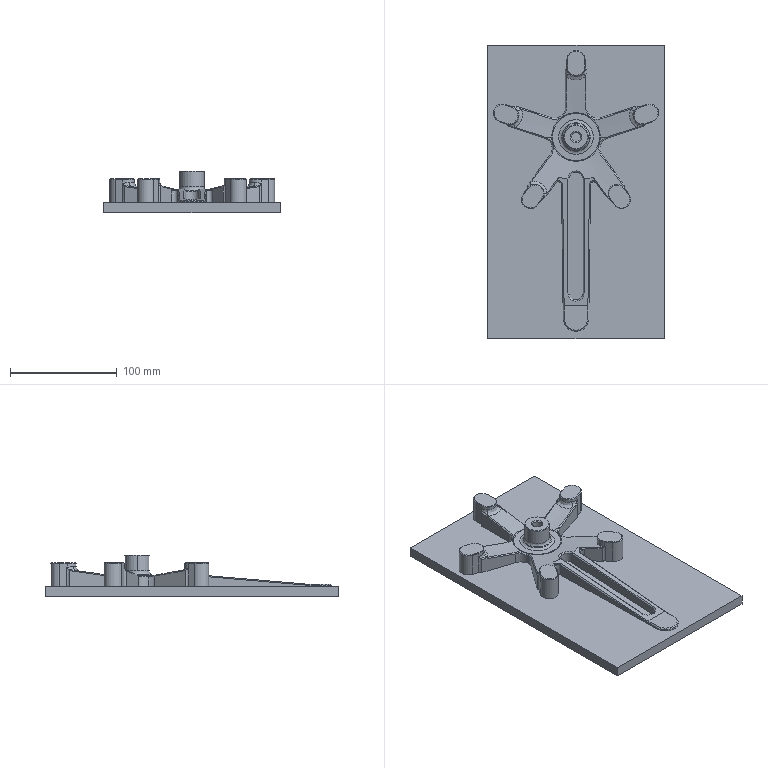NC program | NX | posted with a generic post | part box 165 x 275 x 39 mm
Lines 61374 to 62133 of 70117:
(CONTOUR_AREA , TOOL : D6R3)
N122728 M6
N122730 G54
N122732 G17 G0 G90 X-8.166 Y-25.337 S0 M3
N122734 G43 Z30. H0
N122736 Z-15.6
N122738 G94 G1 Z-15.879 F250.
N122740 X-8.132 Y-25.323 Z-16.661
N122742 X-7.912 Y-25.231 Z-17.407
N122744 X-7.52 Y-25.069 Z-18.066
N122746 X-6.985 Y-24.847 Z-18.592
N122748 X-6.343 Y-24.579 Z-18.951
N122750 X-5.636 Y-24.286 Z-19.118
N122752 X-5.524 Y-24.239 Z-19.128
N122754 X-5.17 Y-24.108 Z-19.157
N122756 X-6.054 Y-23.865 Z-19.162
N122758 X-6.08 Y-23.916 Z-19.154
N122760 X-6.134 Y-24.015 Z-19.139
N122762 X-5.636 Y-24.286 Z-19.118
N122764 X-5.67 Y-24.841 Z-19.038
N122766 X-4.418 Y-24.384 Z-19.139
N122768 X-3.506 Y-24.128 Z-19.197
N122770 X-2.576 Y-23.949 Z-19.239
N122772 X-4.835 Y-23.681 Z-19.228
N122774 X-5.038 Y-23.625 Z-19.229
N122776 X-6.312 Y-23.276 Z-19.235
N122778 X-6.522 Y-23.681 Z-19.171
N122780 X-6.82 Y-24.225 Z-19.084
N122782 X-5.67 Y-24.841 Z-19.038
N122784 X-5.866 Y-25.306 Z-18.967
N122786 X-5.708 Y-25.398 Z-18.959
N122788 X-4.262 Y-24.859 Z-19.075
N122790 X-3.03 Y-24.535 Z-19.148
N122792 X-1.768 Y-24.361 Z-19.191
N122794 X0.969 Y-24.263 Z-19.211
N122796 X2.152 Y-24.397 Z-19.181
N122798 X3.437 Y-24.623 Z-19.128
N122800 X4.684 Y-25.004 Z-19.044
N122802 X5.644 Y-25.399 Z-18.96
N122804 X6.581 Y-24.874 Z-19.002
N122806 X7.544 Y-24.399 Z-19.03
N122808 X7.076 Y-23.547 Z-19.167
N122810 X6.607 Y-22.696 Z-19.304
N122812 X5.938 Y-22.896 Z-19.302
N122814 X4.869 Y-23.088 Z-19.311
N122816 X5.046 Y-24.072 Z-19.166
N122818 X5.05 Y-24.073
N122820 X5.569 Y-24.287 Z-19.12
N122822 X6.163 Y-23.964 Z-19.145
N122824 X6.117 Y-23.88 Z-19.158
N122826 X5.046 Y-24.072 Z-19.166
N122828 X4.957 Y-23.58 Z-19.238
N122830 X2.752 Y-23.976 Z-19.233
N122832 X3.823 Y-24.205 Z-19.179
N122834 X4.867 Y-24.539 Z-19.105
N122836 X5.605 Y-24.843 Z-19.04
N122838 X6.851 Y-24.176 Z-19.089
N122840 X6.363 Y-23.29 Z-19.231
N122842 X6.054 Y-23.383 Z-19.23
N122844 X4.957 Y-23.58 Z-19.238
N122846 X4.869 Y-23.088 Z-19.311
N122848 X2.114 Y-23.582 Z-19.299
N122850 X-0.73 Y-23.633 Z-19.303
N122852 X-2.734 Y-23.411 Z-19.314
N122854 X-4.739 Y-23.189 Z-19.3
N122856 X-6.579 Y-22.685 Z-19.307
N122858 X-7.046 Y-23.566 Z-19.166
N122860 X-7.512 Y-24.447 Z-19.025
N122862 X-5.866 Y-25.306 Z-18.967
N122864 X-6.117 Y-25.738 Z-18.897
N122866 X-5.749 Y-25.957 Z-18.879
N122868 X-4.106 Y-25.335 Z-19.012
N122870 X-2.937 Y-25.027 Z-19.079
N122872 X-1.74 Y-24.86 Z-19.119
N122874 X0.95 Y-24.764 Z-19.139
N122876 X2.096 Y-24.894 Z-19.11
N122878 X3.316 Y-25.108 Z-19.061
N122880 X4.501 Y-25.47 Z-18.983
N122882 X5.687 Y-25.958 Z-18.88
N122884 X6.942 Y-25.25 Z-18.936
N122886 X8.244 Y-24.634 Z-18.966
N122888 X7.547 Y-23.368 Z-19.172
N122890 X6.85 Y-22.101 Z-19.376
N122892 X5.822 Y-22.408 Z-19.374
N122894 X3.945 Y-22.745 Z-19.384
N122896 X2.067 Y-23.082 Z-19.371
N122898 X-0.712 Y-23.134 Z-19.376
N122900 X-1.104 Y-23.117
N122902 X-4.643 Y-22.697 Z-19.372
N122904 X-6.847 Y-22.093 Z-19.378
N122906 X-7.497 Y-23.328 Z-19.179
N122908 X-8.146 Y-24.563 Z-18.981
N122910 X-8.215 Y-24.68 Z-18.962
N122912 X-7.15 Y-25.178 Z-18.938
N122914 X-6.117 Y-25.738 Z-18.897
N122916 X-6.367 Y-26.171 Z-18.828
N122918 X-5.794 Y-26.517 Z-18.798
N122920 X-3.951 Y-25.81 Z-18.947
N122922 X-2.844 Y-25.518 Z-19.01
N122924 X-1.711 Y-25.36 Z-19.047
N122926 X0.93 Y-25.265 Z-19.067
N122928 X2.04 Y-25.391 Z-19.039
N122930 X3.196 Y-25.594 Z-18.993
N122932 X4.319 Y-25.935 Z-18.921
N122934 X5.733 Y-26.517 Z-18.8
N122936 X6.511 Y-26.052 Z-18.84
N122938 X7.31 Y-25.623 Z-18.87
N122940 X8.962 Y-24.879 Z-18.899
N122942 X8.289 Y-23.707 Z-19.091
N122944 X7.616 Y-22.534 Z-19.283
N122946 X7.336 Y-21.956 Z-19.375
N122948 X7.121 Y-21.499 Z-19.448
N122950 X5.706 Y-21.921 Z-19.447
N122952 X3.863 Y-22.252 Z-19.456
N122954 X2.021 Y-22.583 Z-19.444
N122956 X-0.695 Y-22.634 Z-19.448
N122958 X-1.064 Y-22.618
N122960 X-4.547 Y-22.205 Z-19.445
N122962 X-7.121 Y-21.499 Z-19.447
N122964 X-7.327 Y-21.937 Z-19.378
N122966 X-8.646 Y-24.425 Z-18.976
N122968 X-8.908 Y-24.868 Z-18.903
N122970 X-8.941 Y-24.92 Z-18.895
N122972 X-7.631 Y-25.498 Z-18.874
N122974 X-6.367 Y-26.171 Z-18.828
N122976 X-6.618 Y-26.603 Z-18.759
N122978 X-5.842 Y-27.079 Z-18.717
N122980 X-4.609 Y-26.566 Z-18.824
N122982 X-4.273 Y-26.442 Z-18.85
N122984 X-3.795 Y-26.285 Z-18.883
N122986 X-2.751 Y-26.009 Z-18.941
N122988 X-1.682 Y-25.859 Z-18.976
N122990 X0.911 Y-25.766 Z-18.995
N122992 X1.983 Y-25.888 Z-18.969
N122994 X3.076 Y-26.079 Z-18.926
N122996 X4.137 Y-26.401 Z-18.859
N122998 X5.784 Y-27.079 Z-18.719
N123000 X7.052 Y-26.324 Z-18.782
N123002 X8.374 Y-25.669 Z-18.819
N123004 X9.743 Y-25.119 Z-18.827
N123006 X9.059 Y-24.151 Z-18.993
N123008 X7.785 Y-21.738 Z-19.384
N123010 X7.58 Y-21.3 Z-19.453
N123012 X7.385 Y-20.857 Z-19.499
N123014 X6.98 Y-21.019 Z-19.498
N123016 X5.59 Y-21.434
N123018 X4.686 Y-21.596 Z-19.5
N123020 X4.093 Y-21.703
N123022 X3.697 Y-21.774
N123024 X2.878 Y-21.921 Z-19.499
N123026 X1.974 Y-22.083 Z-19.497
N123028 X-0.678 Y-22.134 Z-19.498
N123030 X-1.024 Y-22.12
N123032 X-4.451 Y-21.712 Z-19.497
N123034 X-6.983 Y-21.019 Z-19.498
N123036 X-7.389 Y-20.869
N123038 X-7.578 Y-21.296 Z-19.454
N123040 X-7.777 Y-21.718 Z-19.387
N123042 X-9.015 Y-24.067 Z-19.006
N123044 X-9.334 Y-24.606 Z-18.917
N123046 X-9.693 Y-25.169 Z-18.823
N123048 X-8.123 Y-25.817 Z-18.809
N123050 X-6.618 Y-26.603 Z-18.759
N123052 X-6.869 Y-27.036 Z-18.69
N123054 X-5.884 Y-27.65 Z-18.636
N123056 X-4.108 Y-26.914 Z-18.786
N123058 X-3.639 Y-26.76 Z-18.818
N123060 X-2.657 Y-26.501 Z-18.872
N123062 X-1.652 Y-26.358 Z-18.904
N123064 X0.892 Y-26.267 Z-18.922
N123066 X1.927 Y-26.385 Z-18.898
N123068 X2.956 Y-26.564 Z-18.858
N123070 X3.955 Y-26.867 Z-18.796
N123072 X5.838 Y-27.642 Z-18.638
N123074 X6.574 Y-27.174 Z-18.68
N123076 X7.331 Y-26.741 Z-18.714
N123078 X8.903 Y-25.984 Z-18.751
N123080 X10.538 Y-25.378 Z-18.749
N123082 X10.011 Y-24.632 Z-18.878
N123084 X9.484 Y-23.886 Z-19.007
N123086 X8.235 Y-21.52 Z-19.391
N123088 X7.935 Y-20.869 Z-19.488
N123090 X7.864 Y-20.705 Z-19.498
N123092 X7.846 Y-20.664 Z-19.499
N123094 X7.66 Y-20.208 Z-19.5
N123096 X6.815 Y-20.547
N123098 X5.474 Y-20.947
N123100 X1.928 Y-21.584
N123102 X-0.661 Y-21.634
N123104 X-0.984 Y-21.621
N123106 X-4.355 Y-21.22
N123108 X-6.83 Y-20.542
N123110 X-7.668 Y-20.232
N123112 X-7.799 Y-20.553
N123114 X-7.832 Y-20.633
N123116 X-7.841 Y-20.653
N123118 X-7.849 Y-20.673 Z-19.499
N123120 X-7.866 Y-20.713 Z-19.498
N123122 X-7.935 Y-20.871 Z-19.488
N123124 X-8.227 Y-21.5 Z-19.394
N123126 X-9.449 Y-23.82 Z-19.017
N123128 X-10.466 Y-25.432 Z-18.746
N123130 X-8.625 Y-26.138 Z-18.743
N123132 X-6.869 Y-27.036 Z-18.69
N123134 X-7.12 Y-27.468 Z-18.62
N123136 X-5.917 Y-28.232 Z-18.552
N123138 X-5.557 Y-28.043 Z-18.589
N123140 X-4.243 Y-27.497 Z-18.7
N123142 X-3.943 Y-27.386 Z-18.722
N123144 X-3.483 Y-27.235 Z-18.753
N123146 X-2.564 Y-26.992 Z-18.802
N123148 X-1.622 Y-26.857 Z-18.832
N123150 X0.872 Y-26.768 Z-18.85
N123152 X1.871 Y-26.881 Z-18.827
N123154 X2.836 Y-27.05 Z-18.79
N123156 X3.773 Y-27.333 Z-18.733
N123158 X5.897 Y-28.207 Z-18.556
N123160 X6.742 Y-27.657 Z-18.607
N123162 X7.616 Y-27.156 Z-18.645
N123164 X9.441 Y-26.303 Z-18.682
N123166 X11.35 Y-25.659 Z-18.666
N123168 X10.636 Y-24.652 Z-18.841
N123170 X9.922 Y-23.645 Z-19.015
N123172 X8.685 Y-21.301 Z-19.396
N123174 X8.484 Y-20.872 Z-19.464
N123176 X8.387 Y-20.655 Z-19.492
N123178 X8.34 Y-20.547 Z-19.497
N123180 X8.317 Y-20.492 Z-19.499
N123182 X7.948 Y-19.554 Z-19.5
N123184 X6.65 Y-20.074
N123186 X5.358 Y-20.46
N123188 X1.881 Y-21.084
N123190 X-0.644 Y-21.135
N123192 X-0.944 Y-21.122
N123194 X-4.259 Y-20.728
N123196 X-6.677 Y-20.066
N123198 X-7.958 Y-19.59
N123200 X-8.295 Y-20.444
N123202 X-8.307 Y-20.471
N123204 X-8.318 Y-20.497 Z-19.499
N123206 X-8.341 Y-20.55 Z-19.497
N123208 X-8.387 Y-20.655 Z-19.492
N123210 X-8.481 Y-20.865 Z-19.466
N123212 X-8.676 Y-21.281 Z-19.399
N123214 X-9.884 Y-23.572 Z-19.027
N123216 X-10.954 Y-25.261 Z-18.742
N123218 X-11.277 Y-25.709 Z-18.664
N123220 X-9.844 Y-26.179 Z-18.679
N123222 X-8.455 Y-26.766 Z-18.664
N123224 X-7.12 Y-27.468 Z-18.62
N123226 X-7.371 Y-27.901 Z-18.55
N123228 X-5.955 Y-28.816 Z-18.468
N123230 X-5.344 Y-28.496 Z-18.531
N123232 X-4.06 Y-27.962 Z-18.638
N123234 X-3.778 Y-27.858 Z-18.658
N123236 X-3.327 Y-27.71 Z-18.687
N123238 X-2.47 Y-27.483 Z-18.733
N123240 X-1.592 Y-27.357 Z-18.761
N123242 X0.853 Y-27.269 Z-18.778
N123244 X1.815 Y-27.378 Z-18.755
N123246 X2.716 Y-27.535 Z-18.722
N123248 X3.592 Y-27.799 Z-18.67
N123250 X5.762 Y-28.692 Z-18.492
N123252 X5.926 Y-28.797 Z-18.472
N123254 X6.64 Y-28.311 Z-18.518
N123256 X7.377 Y-27.861 Z-18.556
N123258 X8.913 Y-27.072 Z-18.602
N123260 X10.519 Y-26.437 Z-18.609
N123262 X12.18 Y-25.964 Z-18.576
N123264 X11.263 Y-24.672 Z-18.801
N123266 X10.347 Y-23.38 Z-19.026
N123268 X9.135 Y-21.083 Z-19.4
N123270 X8.886 Y-20.547 Z-19.482
N123272 X8.768 Y-20.277 Z-19.5
N123274 X8.655 Y-20.004
N123276 X8.249 Y-18.895
N123278 X6.485 Y-19.601
N123280 X5.242 Y-19.973
N123282 X1.834 Y-20.584
N123284 X-0.626 Y-20.635
N123286 X-0.904 Y-20.623
N123288 X-4.163 Y-20.236
N123290 X-6.524 Y-19.589
N123292 X-8.252 Y-18.915
N123294 X-8.654 Y-20.003
N123296 X-8.765 Y-20.271
N123298 X-8.772 Y-20.288 Z-19.499
N123300 X-8.779 Y-20.304
N123302 X-8.794 Y-20.338 Z-19.497
N123304 X-8.822 Y-20.404 Z-19.495
N123306 X-8.881 Y-20.537 Z-19.483
N123308 X-9.126 Y-21.062 Z-19.403
N123310 X-10.318 Y-23.324 Z-19.035
N123312 X-11.364 Y-24.975 Z-18.755
N123314 X-12.108 Y-26.009 Z-18.575
N123316 X-10.47 Y-26.485 Z-18.605
N123318 X-8.886 Y-27.117 Z-18.597
N123320 X-7.371 Y-27.901 Z-18.55
N123322 X-7.623 Y-28.334 Z-18.48
N123324 X-5.976 Y-29.423 Z-18.382
N123326 X-5.704 Y-29.249 Z-18.414
N123328 X-5.132 Y-28.949 Z-18.472
N123330 X-3.877 Y-28.428 Z-18.575
N123332 X-3.613 Y-28.33 Z-18.594
N123334 X-3.172 Y-28.185 Z-18.622
N123336 X-2.376 Y-27.974 Z-18.664
N123338 X-1.562 Y-27.856 Z-18.689
N123340 X0.834 Y-27.77 Z-18.706
N123342 X1.758 Y-27.875 Z-18.684
N123344 X2.596 Y-28.021 Z-18.654
N123346 X3.411 Y-28.265 Z-18.606
N123348 X5.53 Y-29.137 Z-18.435
N123350 X5.945 Y-29.404 Z-18.386
N123352 X6.742 Y-28.842 Z-18.44
N123354 X7.57 Y-28.327 Z-18.483
N123356 X9.308 Y-27.443 Z-18.533
N123358 X11.136 Y-26.763 Z-18.531
N123360 X13.029 Y-26.297 Z-18.48
N123362 X10.785 Y-23.139 Z-19.031
N123364 X9.585 Y-20.865 Z-19.402
N123366 X9.314 Y-20.278 Z-19.489
N123368 X9.249 Y-20.13 Z-19.498
N123370 X9.233 Y-20.093 Z-19.499
N123372 G2 X8.566 Y-18.229 R16.959
N123374 G1 X6.321 Y-19.129 Z-19.5
N123376 X5.126 Y-19.486
N123378 X1.788 Y-20.085
N123380 X-0.609 Y-20.135
N123382 X-0.864 Y-20.125
N123384 X-4.067 Y-19.744
N123386 X-6.371 Y-19.113
N123388 X-8.048 Y-18.459
N123390 X-8.562 Y-18.229
N123392 X-8.624 Y-18.439
N123394 X-9.054 Y-19.659
N123396 X-9.215 Y-20.052
N123398 X-9.223 Y-20.071
N123400 X-9.239 Y-20.108 Z-19.498
N123402 X-9.304 Y-20.256 Z-19.492
N123404 X-9.576 Y-20.844 Z-19.406
N123406 X-10.752 Y-23.076 Z-19.041
N123408 X-11.774 Y-24.688 Z-18.768
N123410 X-12.96 Y-26.337 Z-18.479
N123412 X-11.11 Y-26.801 Z-18.528
N123414 X-9.324 Y-27.47
N123416 X-7.623 Y-28.334 Z-18.48
N123418 X-7.874 Y-28.767 Z-18.411
N123420 X-6.916 Y-29.368 Z-18.361
N123422 X-6.001 Y-30.034 Z-18.295
N123424 X-5.452 Y-29.681 Z-18.36
N123426 X-4.92 Y-29.403 Z-18.413
N123428 X-3.016 Y-28.66 Z-18.556
N123430 X-2.282 Y-28.465 Z-18.594
N123432 X-1.531 Y-28.355 Z-18.617
N123434 X0.814 Y-28.271 Z-18.633
N123436 X1.702 Y-28.372 Z-18.613
N123438 X2.477 Y-28.506 Z-18.586
N123440 X3.23 Y-28.731 Z-18.543
N123442 X5.298 Y-29.582 Z-18.378
N123444 X5.969 Y-30.014 Z-18.299
N123446 X6.67 Y-29.496 Z-18.351
N123448 X7.396 Y-29.016 Z-18.394
N123450 X8.921 Y-28.173 Z-18.45
N123452 X10.525 Y-27.495 Z-18.466
N123454 X12.192 Y-26.989 Z-18.441
N123456 X13.902 Y-26.662 Z-18.376
N123458 X11.21 Y-22.873 Z-19.039
N123460 X10.034 Y-20.646 Z-19.403
N123462 X9.772 Y-20.078 Z-19.488
N123464 X9.709 Y-19.934 Z-19.497
N123466 X9.679 Y-19.862 Z-19.5
N123468 X9.53 Y-19.499
N123470 X9.115 Y-18.317
N123472 X8.876 Y-17.518
N123474 X8.627 Y-17.666
N123476 X6.156 Y-18.656
N123478 X5.01 Y-18.998
N123480 X1.741 Y-19.585
N123482 X-0.592 Y-19.636
N123484 X-0.824 Y-19.626
N123486 X-3.97 Y-19.252
N123488 X-6.218 Y-18.636
N123490 X-7.546 Y-18.136
N123492 X-8.872 Y-17.516
N123494 G2 X-9.676 Y-19.858 R17.69
N123496 G1 X-9.684 Y-19.876 Z-19.499
N123498 X-9.699 Y-19.912 Z-19.498
N123500 X-9.762 Y-20.056 Z-19.491
N123502 X-10.025 Y-20.625 Z-19.406
N123504 X-11.187 Y-22.829 Z-19.047
N123506 X-12.184 Y-24.402 Z-18.779
N123508 X-13.839 Y-26.696 Z-18.375
N123510 X-12.28 Y-26.996 Z-18.435
N123512 X-10.757 Y-27.444 Z-18.461
N123514 X-9.284 Y-28.036 Z-18.453
N123516 X-7.874 Y-28.767 Z-18.411
N123518 X-8.125 Y-29.199 Z-18.341
N123520 X-7.05 Y-29.882 Z-18.284
N123522 X-6.032 Y-30.648 Z-18.207
N123524 X-5.201 Y-30.114 Z-18.305
N123526 X-4.707 Y-29.856 Z-18.353
N123528 X-2.86 Y-29.135 Z-18.49
N123530 X-2.188 Y-28.956 Z-18.524
N123532 X-1.499 Y-28.854 Z-18.545
N123534 X0.795 Y-28.772 Z-18.561
N123536 X1.646 Y-28.869 Z-18.542
N123538 X2.357 Y-28.992 Z-18.517
N123540 X3.049 Y-29.198 Z-18.478
N123542 X5.065 Y-30.027 Z-18.32
N123544 X6.001 Y-30.629 Z-18.21
N123546 X6.765 Y-30.042 Z-18.271
N123548 X7.563 Y-29.501 Z-18.32
N123550 X9.25 Y-28.569 Z-18.381
N123552 X11.036 Y-27.846 Z-18.392
N123554 X12.895 Y-27.342 Z-18.352
N123556 X14.802 Y-27.065 Z-18.263
N123558 X11.634 Y-22.607 Z-19.046
N123560 X10.484 Y-20.428 Z-19.402
N123562 X10.23 Y-19.877 Z-19.485
N123564 X10.169 Y-19.738 Z-19.496
N123566 X10.139 Y-19.668 Z-19.499
N123568 G2 X9.171 Y-16.76 R19.731
N123570 G1 X8.404 Y-17.217 Z-19.5
N123572 X5.991 Y-18.184
N123574 X4.894 Y-18.511
N123576 X1.695 Y-19.085
N123578 X-0.784 Y-19.127
N123580 X-3.874 Y-18.76
N123582 X-6.065 Y-18.16
N123584 X-7.345 Y-17.678
N123586 X-8.461 Y-17.179
N123588 X-9.168 Y-16.758
N123590 X-9.581 Y-18.148
N123592 X-9.985 Y-19.294
N123594 X-10.122 Y-19.628
N123596 X-10.129 Y-19.646 Z-19.499
N123598 X-10.159 Y-19.716 Z-19.497
N123600 X-10.22 Y-19.855 Z-19.488
N123602 X-10.475 Y-20.406 Z-19.406
N123604 X-11.621 Y-22.581 Z-19.05
N123606 X-12.594 Y-24.116 Z-18.789
N123608 X-13.67 Y-25.605 Z-18.526
N123610 X-14.746 Y-27.094 Z-18.263
N123612 X-13.014 Y-27.345 Z-18.344
N123614 X-11.32 Y-27.784 Z-18.385
N123616 X-9.684 Y-28.404 Z-18.384
N123618 X-8.125 Y-29.199 Z-18.341
N123620 X-8.377 Y-29.632 Z-18.271
N123622 X-7.182 Y-30.401 Z-18.207
N123624 X-6.062 Y-31.275 Z-18.117
N123626 X-5.929 Y-31.176 Z-18.135
N123628 X-4.949 Y-30.547 Z-18.249
N123630 X-4.495 Y-30.309 Z-18.293
N123632 X-2.704 Y-29.61 Z-18.424
N123634 X-2.093 Y-29.447 Z-18.455
N123636 X-1.467 Y-29.353 Z-18.474
N123638 X0.776 Y-29.273 Z-18.489
N123640 X1.589 Y-29.365 Z-18.471
N123642 X2.238 Y-29.477 Z-18.449
N123644 X2.869 Y-29.664 Z-18.414
N123646 X4.833 Y-30.472 Z-18.262
N123648 X5.927 Y-31.176 Z-18.135
N123650 X6.032 Y-31.254 Z-18.121
N123652 X6.719 Y-30.699 Z-18.18
N123654 X7.436 Y-30.182 Z-18.229
N123656 X8.952 Y-29.277 Z-18.297
N123658 X10.562 Y-28.549 Z-18.322
N123660 X12.243 Y-28.008 Z-18.304
N123662 X13.975 Y-27.661 Z-18.242
N123664 X15.735 Y-27.513 Z-18.141
N123666 X12.072 Y-22.367 Z-19.048
N123668 X10.934 Y-20.21 Z-19.4
N123670 X10.688 Y-19.676 Z-19.481
N123672 X10.572 Y-19.406 Z-19.5
N123674 X10.461 Y-19.134
N123676 X10.071 Y-18.026
N123678 X9.601 Y-16.453
N123680 X9.475 Y-15.997
N123682 X8.182 Y-16.767
N123684 X5.826 Y-17.711
N123686 X4.777 Y-18.024
N123688 X1.648 Y-18.586
N123690 X-0.744 Y-18.628
N123692 X-3.778 Y-18.268
N123694 X-5.912 Y-17.683
N123696 X-7.145 Y-17.22
N123698 X-8.23 Y-16.734
N123700 X-9.473 Y-15.996
N123702 G2 X-10.569 Y-19.401 R27.65
N123704 G1 X-10.576 Y-19.418 Z-19.499
N123706 X-10.677 Y-19.654 Z-19.484
N123708 X-10.925 Y-20.188 Z-19.403
N123710 X-12.056 Y-22.333 Z-19.053
N123712 X-13.004 Y-23.829 Z-18.798
N123714 X-14.345 Y-25.683 Z-18.469
N123716 X-15.686 Y-27.537 Z-18.141
N123718 X-14.728 Y-27.597 Z-18.2
N123720 X-13.775 Y-27.717 Z-18.248
N123722 X-12.832 Y-27.895 Z-18.284
N123724 X-11.901 Y-28.131 Z-18.307
N123726 X-10.987 Y-28.423 Z-18.317
N123728 X-10.092 Y-28.772 Z-18.315
N123730 X-9.221 Y-29.175 Z-18.299
N123732 X-8.377 Y-29.632 Z-18.271
N123734 X-8.628 Y-30.064 Z-18.201
N123736 X-7.304 Y-30.929 Z-18.128
N123738 X-6.079 Y-31.927 Z-18.024
N123740 X-5.94 Y-31.808 Z-18.045
N123742 X-5.644 Y-31.587 Z-18.084
N123744 X-4.698 Y-30.98 Z-18.193
N123746 X-4.283 Y-30.762 Z-18.233
N123748 X-2.548 Y-30.086 Z-18.358
N123750 X-1.998 Y-29.938 Z-18.385
N123752 X-1.434 Y-29.853 Z-18.402
N123754 X0.756 Y-29.774 Z-18.417
N123756 X1.533 Y-29.862 Z-18.4
N123758 X2.119 Y-29.963 Z-18.38
N123760 X2.69 Y-30.131 Z-18.349
N123762 X4.601 Y-30.917 Z-18.204
N123764 X5.642 Y-31.587 Z-18.084
N123766 X5.932 Y-31.803 Z-18.046
N123768 X6.051 Y-31.905 Z-18.028
N123770 X7.341 Y-30.859 Z-18.137
N123772 X8.739 Y-29.962 Z-18.21
N123774 X10.227 Y-29.225 Z-18.246
N123776 X11.787 Y-28.656 Z-18.243
N123778 X13.4 Y-28.262 Z-18.201
N123780 X15.047 Y-28.049 Z-18.121
N123782 X16.708 Y-28.018 Z-18.007
N123784 X12.497 Y-22.101 Z-19.051
N123786 X11.384 Y-19.992 Z-19.396
N123788 X11.146 Y-19.476 Z-19.476
N123790 X11.034 Y-19.215 Z-19.497
N123792 X11.007 Y-19.149 Z-19.5
N123794 X10.927 Y-18.951
N123796 X10.55 Y-17.88
N123798 X10.081 Y-16.313
N123800 X9.805 Y-15.219
N123802 X7.96 Y-16.318
N123804 X5.661 Y-17.238
N123806 X4.661 Y-17.537
N123808 X1.602 Y-18.086
N123810 X-0.704 Y-18.13
N123812 X-3.682 Y-17.776
N123814 X-5.759 Y-17.207
N123816 X-6.944 Y-16.762
N123818 X-8. Y-16.289
N123820 X-9.803 Y-15.218
N123822 G2 X-11.01 Y-19.159 R27.18
N123824 G1 X-11.023 Y-19.192 Z-19.498
N123826 X-11.135 Y-19.453 Z-19.479
N123828 X-11.374 Y-19.969 Z-19.399
N123830 X-12.49 Y-22.086 Z-19.054
N123832 X-13.414 Y-23.543 Z-18.805
N123834 X-15.04 Y-25.79 Z-18.406
N123836 X-16.666 Y-28.037 Z-18.008
N123838 X-14.988 Y-28.077 Z-18.121
N123840 X-13.324 Y-28.303 Z-18.2
N123842 X-11.696 Y-28.714 Z-18.24
N123844 X-10.124 Y-29.303
N123846 X-8.628 Y-30.064 Z-18.201
N123848 X-8.879 Y-30.496 Z-18.131
N123850 X-7.422 Y-31.464 Z-18.049
N123852 X-6.092 Y-32.599 Z-17.929
N123854 X-5.359 Y-31.998 Z-18.032
N123856 X-4.446 Y-31.412 Z-18.136
N123858 X-4.07 Y-31.215 Z-18.172
N123860 X-2.393 Y-30.561 Z-18.291
N123862 X-1.401 Y-30.352 Z-18.33
N123864 X0.737 Y-30.275 Z-18.344
N123866 X1.477 Y-30.359 Z-18.328
N123868 X2.001 Y-30.449 Z-18.311
N123870 X2.511 Y-30.598 Z-18.284
N123872 X4.369 Y-31.363 Z-18.145
N123874 X5.358 Y-31.999 Z-18.032
N123876 X5.62 Y-32.194 Z-17.998
N123878 X6.065 Y-32.575 Z-17.933
N123880 X6.74 Y-31.966 Z-18.
N123882 X7.451 Y-31.399 Z-18.057
N123884 X8.972 Y-30.405 Z-18.14
N123886 X10.605 Y-29.608 Z-18.176
N123888 X12.325 Y-29.021 Z-18.164
N123890 X14.104 Y-28.653 Z-18.106
N123892 X15.916 Y-28.51 Z-18.002
N123894 X17.731 Y-28.594 Z-17.859
N123896 X12.921 Y-21.834 Z-19.054
N123898 X11.834 Y-19.773 Z-19.39
N123900 X11.604 Y-19.275 Z-19.469
N123902 X11.496 Y-19.023 Z-19.495
N123904 X11.443 Y-18.896 Z-19.5
N123906 G2 X10.164 Y-14.423 R26.412
N123908 G1 X7.737 Y-15.868
N123910 X5.496 Y-16.766
N123912 X4.545 Y-17.05
N123914 X1.555 Y-17.587
N123916 X-0.663 Y-17.631
N123918 X-3.586 Y-17.284
N123920 X-5.606 Y-16.73
N123922 X-6.744 Y-16.304
N123924 X-7.769 Y-15.845
N123926 X-10.162 Y-14.423
N123928 G2 X-11.439 Y-18.89 R25.645
N123930 G1 X-11.446 Y-18.905
N123932 X-11.459 Y-18.937 Z-19.498
N123934 X-11.485 Y-19.001 Z-19.496
N123936 X-11.593 Y-19.253 Z-19.472
N123938 X-11.824 Y-19.75 Z-19.394
N123940 X-12.924 Y-21.838 Z-19.053
N123942 X-13.824 Y-23.257 Z-18.811
N123944 X-15.761 Y-25.932 Z-18.335
N123946 X-17.699 Y-28.608 Z-17.86
N123948 X-15.868 Y-28.533 Z-18.003
N123950 X-14.041 Y-28.688 Z-18.105
N123952 X-12.249 Y-29.071 Z-18.162
N123954 X-10.519 Y-29.677 Z-18.171
N123956 X-8.879 Y-30.496 Z-18.131
N123958 X-9.13 Y-30.929 Z-18.061
N123960 X-8.044 Y-31.628 Z-18.005
N123962 X-7.026 Y-32.425 Z-17.927
N123964 X-6.086 Y-33.311 Z-17.828
N123966 X-5.314 Y-32.589 Z-17.949
N123968 X-5.074 Y-32.41 Z-17.98
N123970 X-4.194 Y-31.845 Z-18.079
N123972 X-2.624 Y-31.163 Z-18.202
N123974 X-2.237 Y-31.036 Z-18.224
N123976 X-1.366 Y-30.851 Z-18.258
N123978 X0.718 Y-30.776 Z-18.272
N123980 X1.421 Y-30.856 Z-18.257
N123982 X2.333 Y-31.065 Z-18.219
N123984 X4.136 Y-31.808 Z-18.086
N123986 X5.073 Y-32.41 Z-17.98
N123988 X5.308 Y-32.585 Z-17.95
N123990 X6.064 Y-33.283 Z-17.832
N123992 X6.689 Y-32.676 Z-17.901
N123994 X7.35 Y-32.109 Z-17.961
N123996 X8.773 Y-31.104 Z-18.051
N123998 X10.308 Y-30.282 Z-18.098
N124000 X11.934 Y-29.657 Z-18.101
N124002 X13.624 Y-29.238 Z-18.06
N124004 X15.353 Y-29.031 Z-17.975
N124006 X17.095 Y-29.039 Z-17.851
N124008 X18.822 Y-29.264 Z-17.693
N124010 X13.359 Y-21.594 Z-19.051
N124012 X12.284 Y-19.555 Z-19.383
N124014 X12.062 Y-19.075 Z-19.459
N124016 X11.957 Y-18.831 Z-19.49
N124018 X11.907 Y-18.709 Z-19.497
N124020 X11.882 Y-18.648 Z-19.499
N124022 G2 X11.04 Y-16.032 R19.798
N124024 G1 X10.659 Y-14.355 Z-19.5
N124026 X10.525 Y-13.533
N124028 X9.908 Y-13.993
N124030 X7.515 Y-15.418
N124032 X5.332 Y-16.293
N124034 X4.429 Y-16.563
N124036 X1.508 Y-17.087
N124038 X1.333 Y-17.088
N124040 X-0.623 Y-17.132
N124042 X-3.49 Y-16.791
N124044 X-5.453 Y-16.254
N124046 X-6.543 Y-15.846
N124048 X-7.538 Y-15.4
N124050 X-9.915 Y-13.988
N124052 X-10.524 Y-13.534
N124054 X-10.658 Y-14.355
N124056 X-11.026 Y-15.987
N124058 X-11.495 Y-17.567
N124060 X-11.865 Y-18.61
N124062 X-11.872 Y-18.625
N124064 X-11.896 Y-18.687 Z-19.498
N124066 X-11.947 Y-18.809 Z-19.493
N124068 X-12.051 Y-19.052 Z-19.463
N124070 X-12.273 Y-19.532 Z-19.387
N124072 X-13.359 Y-21.59 Z-19.051
N124074 X-14.234 Y-22.97 Z-18.815
N124076 X-18.802 Y-29.275 Z-17.693
N124078 X-17.146 Y-29.062 Z-17.845
N124080 X-15.476 Y-29.047 Z-17.965
N124082 X-13.817 Y-29.23 Z-18.049
N124084 X-12.191 Y-29.609 Z-18.094
N124086 X-10.621 Y-30.177 Z-18.098
N124088 X-9.13 Y-30.929 Z-18.061
N124090 X-9.381 Y-31.361 Z-17.99
N124092 X-8.189 Y-32.14 Z-17.928
N124094 X-7.086 Y-33.039 Z-17.838
N124096 X-6.082 Y-34.05 Z-17.723
N124098 X-5.572 Y-33.489 Z-17.815
N124100 X-5.406 Y-33.327 Z-17.842
N124102 X-5.001 Y-32.979 Z-17.901
N124104 X-4.789 Y-32.821 Z-17.928
N124106 X-3.943 Y-32.278 Z-18.022
N124108 X-3.646 Y-32.122 Z-18.049
N124110 X-2.081 Y-31.511 Z-18.157
N124112 X-1.331 Y-31.35 Z-18.186
N124114 X0.698 Y-31.277 Z-18.2
N124116 X1.364 Y-31.353 Z-18.186
N124118 X2.155 Y-31.533 Z-18.153
N124120 X3.904 Y-32.253 Z-18.026
N124122 X4.788 Y-32.821 Z-17.928
N124124 X4.995 Y-32.976 Z-17.901
N124126 X5.419 Y-33.339 Z-17.84
N124128 X5.594 Y-33.508 Z-17.812
N124130 X6.058 Y-34.023 Z-17.727
N124132 X7.268 Y-32.83 Z-17.862
N124134 X8.618 Y-31.798 Z-17.96
N124136 X10.086 Y-30.943 Z-18.018
N124138 X11.65 Y-30.279 Z-18.033
N124140 X13.285 Y-29.815 Z-18.004
N124142 X14.965 Y-29.56 Z-17.933
N124144 X16.663 Y-29.517 Z-17.823
N124146 X18.354 Y-29.688 Z-17.677
N124148 X20.01 Y-30.068 Z-17.502
N124150 X13.798 Y-21.353 Z-19.046
N124152 X12.733 Y-19.337 Z-19.374
N124154 X12.52 Y-18.874 Z-19.447
N124156 X12.323 Y-18.404 Z-19.498
N124158 X12.312 Y-18.374 Z-19.499
N124160 G2 X10.903 Y-12.573 R25.107
N124162 G1 X9.65 Y-13.565 Z-19.5
N124164 X7.293 Y-14.969
N124166 X5.167 Y-15.821
N124168 X4.313 Y-16.075
N124170 X1.462 Y-16.587
N124172 X1.317 Y-16.588
N124174 X-0.583 Y-16.633
N124176 X-3.394 Y-16.299
N124178 X-5.3 Y-15.777
N124180 X-6.343 Y-15.388
N124182 X-7.308 Y-14.956
N124184 X-9.638 Y-13.571
N124186 X-10.593 Y-12.84
N124188 X-10.898 Y-12.545
N124190 G2 X-12.301 Y-18.352 R23.85
N124192 G1 X-12.313 Y-18.381 Z-19.499
N124194 X-12.509 Y-18.851 Z-19.451
N124196 X-12.723 Y-19.313 Z-19.378
N124198 X-13.793 Y-21.342 Z-19.048
N124200 X-14.644 Y-22.684 Z-18.819
N124202 X-20.005 Y-30.08 Z-17.501
N124204 X-18.475 Y-29.724 Z-17.663
N124206 X-16.914 Y-29.549 Z-17.801
N124208 X-15.344 Y-29.555 Z-17.909
N124210 X-13.784 Y-29.743 Z-17.984
N124212 X-12.257 Y-30.111 Z-18.023
N124214 X-10.783 Y-30.652 Z-18.025
N124216 X-9.381 Y-31.361 Z-17.99
N124218 X-9.632 Y-31.793 Z-17.92
N124220 X-8.33 Y-32.658 Z-17.851
N124222 X-7.141 Y-33.671 Z-17.747
N124224 X-6.082 Y-34.82 Z-17.618
N124226 X-5.069 Y-33.696 Z-17.807
N124228 X-4.688 Y-33.369 Z-17.864
N124230 X-4.504 Y-33.232 Z-17.888
N124232 X-3.691 Y-32.71 Z-17.982
N124234 X-3.433 Y-32.575 Z-18.007
N124236 X-1.925 Y-31.986 Z-18.114
N124238 X-1.294 Y-31.849 Z-18.141
N124240 X0.679 Y-31.778 Z-18.157